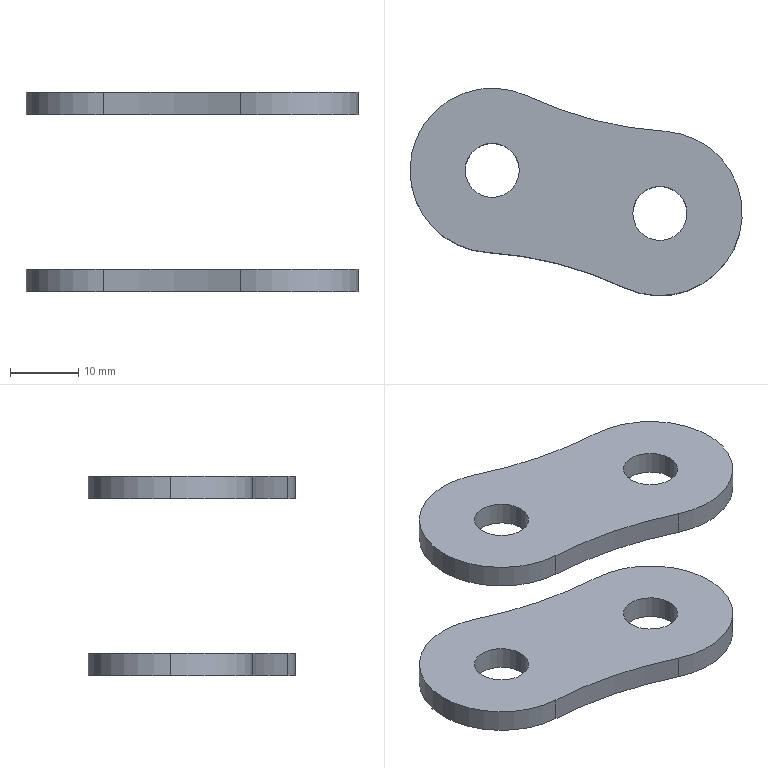Part | STEP file | 2 solids | 22 faces | box 48.732 x 30.447 x 29.29 mm | volume 6239 mm3 | cylinder 18 | plane 4 | commonest cylinder face diameters 7.94 x8 24.13 x6 110.761 x4